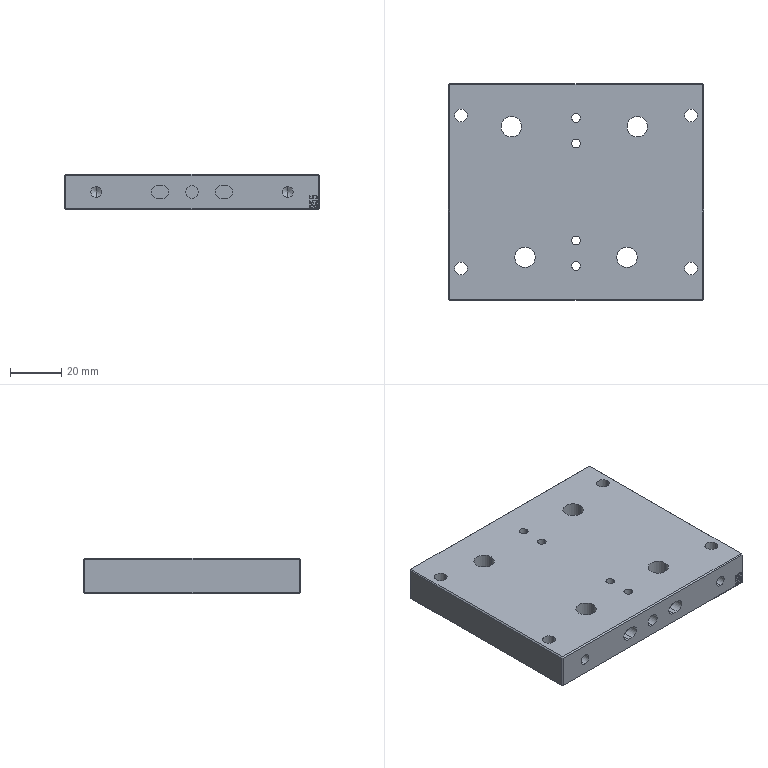Part | SolidWorks | features BaseBody 1 | 1 solid | 217 faces | box 100 x 85 x 14 mm | volume 103040 mm3 | plane 101 | cylinder 64 | spline 44 | cone 8 | commonest cylinder face diameters 5 x24 3.4 x8 4.2 x8 6 x8 8 x8 21 x8